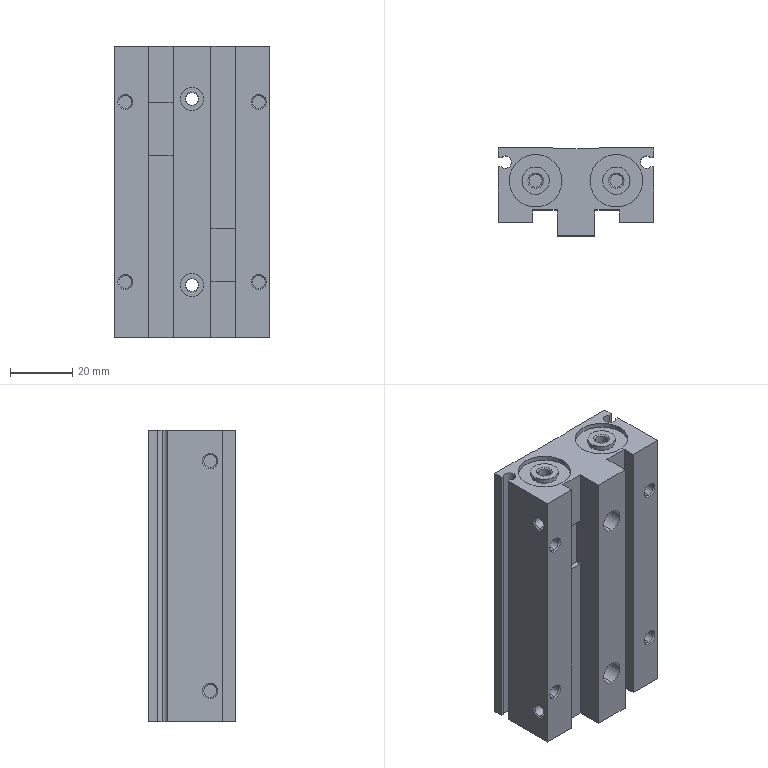Part | STEP file | MHF2-16D1_32-01-CC | 1 solid | 132 faces | box 50 x 28.3 x 94 mm | volume 105067 mm3 | plane 56 | cylinder 52 | cone 24 | commonest cylinder face diameters 4.134 x24 4 x8 17 x8 4.3 x4 7.5 x4 8.8 x4